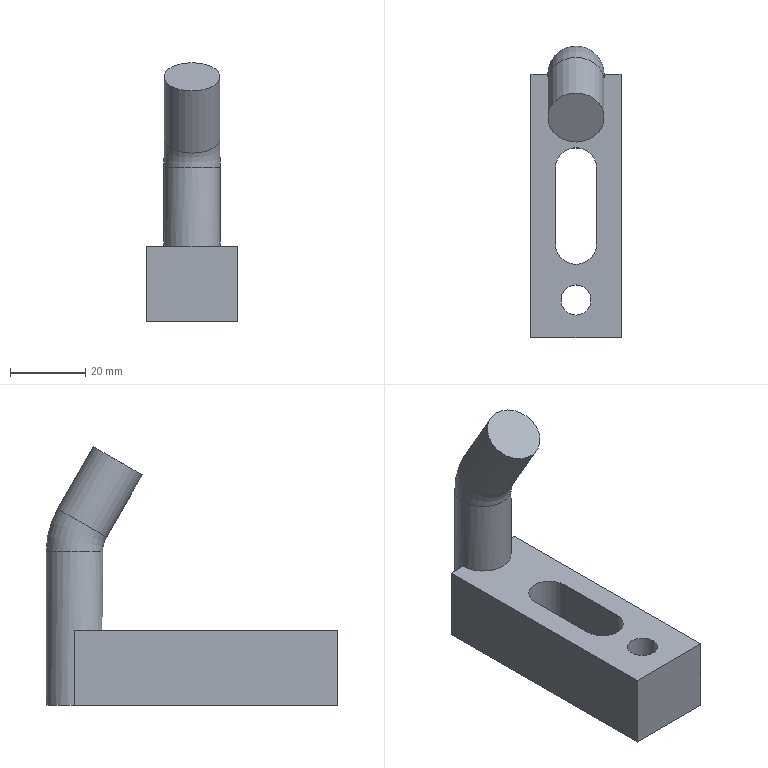Part | NX | features solid 2 | 1 solid | 16 faces | box 24 x 77.5 x 68.75 mm | volume 36527 mm3 | plane 10 | cylinder 5 | torus 1 | commonest cylinder face diameters 11 x2 15 x2 8 x1
STEP:
#1=CARTESIAN_POINT('',(-340.,270.,5.));
#2=VERTEX_POINT('',#1);
#3=CARTESIAN_POINT('',(-340.,266.,5.));
#4=DIRECTION('',(0.,0.,-1.));
#5=DIRECTION('',(0.,1.,0.));
#6=AXIS2_PLACEMENT_3D('',#3,#4,#5);
#7=CIRCLE('',#6,4.);
#8=EDGE_CURVE('',#2,#2,#7,.T.);
#9=ORIENTED_EDGE('',*,*,#8,.T.);
#10=EDGE_LOOP('',(#9));
#11=FACE_BOUND('',#10,.T.);
#12=CARTESIAN_POINT('',(-334.5,301.,5.));
#13=VERTEX_POINT('',#12);
#14=CARTESIAN_POINT('',(-334.5,281.,5.));
#15=VERTEX_POINT('',#14);
#16=CARTESIAN_POINT('',(-334.5,291.,5.));
#17=DIRECTION('',(0.,-1.,0.));
#18=VECTOR('',#17,1000.);
#19=LINE('',#16,#18);
#20=EDGE_CURVE('',#13,#15,#19,.T.);
#21=ORIENTED_EDGE('',*,*,#20,.T.);
#22=CARTESIAN_POINT('',(-345.5,281.,5.));
#23=VERTEX_POINT('',#22);
#24=CARTESIAN_POINT('',(-340.,281.,5.));
#25=DIRECTION('',(0.,0.,1.));
#26=DIRECTION('',(0.,-1.,0.));
#27=AXIS2_PLACEMENT_3D('',#24,#25,#26);
#28=CIRCLE('',#27,5.5);
#29=EDGE_CURVE('',#23,#15,#28,.T.);
#30=ORIENTED_EDGE('',*,*,#29,.F.);
#31=CARTESIAN_POINT('',(-345.5,301.,5.));
#32=VERTEX_POINT('',#31);
#33=CARTESIAN_POINT('',(-345.5,291.,5.));
#34=DIRECTION('',(0.,-1.,0.));
#35=VECTOR('',#34,1000.);
#36=LINE('',#33,#35);
#37=EDGE_CURVE('',#32,#23,#36,.T.);
#38=ORIENTED_EDGE('',*,*,#37,.F.);
#39=CARTESIAN_POINT('',(-340.,301.,5.));
#40=DIRECTION('',(0.,0.,1.));
#41=DIRECTION('',(0.,-1.,0.));
#42=AXIS2_PLACEMENT_3D('',#39,#40,#41);
#43=CIRCLE('',#42,5.5);
#44=EDGE_CURVE('',#13,#32,#43,.T.);
#45=ORIENTED_EDGE('',*,*,#44,.F.);
#46=EDGE_LOOP('',(#21,#30,#38,#45));
#47=FACE_BOUND('',#46,.T.);
#48=CARTESIAN_POINT('',(-328.,326.,5.));
#49=VERTEX_POINT('',#48);
#50=CARTESIAN_POINT('',(-332.5,326.,5.));
#51=VERTEX_POINT('',#50);
#52=CARTESIAN_POINT('',(-328.,326.,5.));
#53=DIRECTION('',(-1.,0.,0.));
#54=VECTOR('',#53,1000.);
#55=LINE('',#52,#54);
#56=EDGE_CURVE('',#49,#51,#55,.T.);
#57=ORIENTED_EDGE('',*,*,#56,.T.);
#58=CARTESIAN_POINT('',(-347.5,326.,5.));
#59=VERTEX_POINT('',#58);
#60=CARTESIAN_POINT('',(-340.,326.,5.));
#61=DIRECTION('',(0.,0.,1.));
#62=DIRECTION('',(1.,0.,0.));
#63=AXIS2_PLACEMENT_3D('',#60,#61,#62);
#64=CIRCLE('',#63,7.5);
#65=EDGE_CURVE('',#51,#59,#64,.F.);
#66=ORIENTED_EDGE('',*,*,#65,.T.);
#67=CARTESIAN_POINT('',(-352.,326.,5.));
#68=VERTEX_POINT('',#67);
#69=CARTESIAN_POINT('',(-328.,326.,5.));
#70=DIRECTION('',(-1.,0.,0.));
#71=VECTOR('',#70,1000.);
#72=LINE('',#69,#71);
#73=EDGE_CURVE('',#59,#68,#72,.T.);
#74=ORIENTED_EDGE('',*,*,#73,.T.);
#75=CARTESIAN_POINT('',(-352.,256.,5.));
#76=VERTEX_POINT('',#75);
#77=CARTESIAN_POINT('',(-352.,326.,5.));
#78=DIRECTION('',(0.,-1.,0.));
#79=VECTOR('',#78,1000.);
#80=LINE('',#77,#79);
#81=EDGE_CURVE('',#68,#76,#80,.T.);
#82=ORIENTED_EDGE('',*,*,#81,.T.);
#83=CARTESIAN_POINT('',(-328.,256.,5.));
#84=VERTEX_POINT('',#83);
#85=CARTESIAN_POINT('',(-352.,256.,5.));
#86=DIRECTION('',(1.,0.,0.));
#87=VECTOR('',#86,1000.);
#88=LINE('',#85,#87);
#89=EDGE_CURVE('',#76,#84,#88,.T.);
#90=ORIENTED_EDGE('',*,*,#89,.T.);
#91=CARTESIAN_POINT('',(-328.,256.,5.));
#92=DIRECTION('',(0.,1.,0.));
#93=VECTOR('',#92,1000.);
#94=LINE('',#91,#93);
#95=EDGE_CURVE('',#84,#49,#94,.T.);
#96=ORIENTED_EDGE('',*,*,#95,.T.);
#97=EDGE_LOOP('',(#57,#66,#74,#82,#90,#96));
#98=FACE_BOUND('',#97,.T.);
#99=CARTESIAN_POINT('',(-328.,256.,5.));
#100=DIRECTION('',(0.,0.,1.));
#101=DIRECTION('',(0.,-1.,0.));
#102=AXIS2_PLACEMENT_3D('',#99,#100,#101);
#103=PLANE('',#102);
#104=ADVANCED_FACE('',(#11,#47,#98),#103,.T.);
#105=CARTESIAN_POINT('',(-347.5,326.,-15.));
#106=VERTEX_POINT('',#105);
#107=CARTESIAN_POINT('',(-352.,326.,-15.));
#108=VERTEX_POINT('',#107);
#109=CARTESIAN_POINT('',(-328.,326.,-15.));
#110=DIRECTION('',(-1.,0.,0.));
#111=VECTOR('',#110,1000.);
#112=LINE('',#109,#111);
#113=EDGE_CURVE('',#106,#108,#112,.T.);
#114=ORIENTED_EDGE('',*,*,#113,.F.);
#115=CARTESIAN_POINT('',(-332.5,326.,-15.));
#116=VERTEX_POINT('',#115);
#117=CARTESIAN_POINT('',(-340.,326.,-15.));
#118=DIRECTION('',(0.,0.,1.));
#119=DIRECTION('',(0.,-1.,0.));
#120=AXIS2_PLACEMENT_3D('',#117,#118,#119);
#121=CIRCLE('',#120,7.5);
#122=EDGE_CURVE('',#116,#106,#121,.T.);
#123=ORIENTED_EDGE('',*,*,#122,.F.);
#124=CARTESIAN_POINT('',(-328.,326.,-15.));
#125=VERTEX_POINT('',#124);
#126=CARTESIAN_POINT('',(-328.,326.,-15.));
#127=DIRECTION('',(-1.,0.,0.));
#128=VECTOR('',#127,1000.);
#129=LINE('',#126,#128);
#130=EDGE_CURVE('',#125,#116,#129,.T.);
#131=ORIENTED_EDGE('',*,*,#130,.F.);
#132=CARTESIAN_POINT('',(-328.,256.,-15.));
#133=VERTEX_POINT('',#132);
#134=CARTESIAN_POINT('',(-328.,256.,-15.));
#135=DIRECTION('',(0.,1.,0.));
#136=VECTOR('',#135,1000.);
#137=LINE('',#134,#136);
#138=EDGE_CURVE('',#133,#125,#137,.T.);
#139=ORIENTED_EDGE('',*,*,#138,.F.);
#140=CARTESIAN_POINT('',(-352.,256.,-15.));
#141=VERTEX_POINT('',#140);
#142=CARTESIAN_POINT('',(-352.,256.,-15.));
#143=DIRECTION('',(1.,0.,0.));
#144=VECTOR('',#143,1000.);
#145=LINE('',#142,#144);
#146=EDGE_CURVE('',#141,#133,#145,.T.);
#147=ORIENTED_EDGE('',*,*,#146,.F.);
#148=CARTESIAN_POINT('',(-352.,326.,-15.));
#149=DIRECTION('',(0.,-1.,0.));
#150=VECTOR('',#149,1000.);
#151=LINE('',#148,#150);
#152=EDGE_CURVE('',#108,#141,#151,.T.);
#153=ORIENTED_EDGE('',*,*,#152,.F.);
#154=EDGE_LOOP('',(#114,#123,#131,#139,#147,#153));
#155=FACE_BOUND('',#154,.T.);
#156=CARTESIAN_POINT('',(-345.5,281.,-15.));
#157=VERTEX_POINT('',#156);
#158=CARTESIAN_POINT('',(-334.5,281.,-15.));
#159=VERTEX_POINT('',#158);
#160=CARTESIAN_POINT('',(-340.,281.,-15.));
#161=DIRECTION('',(0.,0.,1.));
#162=DIRECTION('',(0.,-1.,0.));
#163=AXIS2_PLACEMENT_3D('',#160,#161,#162);
#164=CIRCLE('',#163,5.5);
#165=EDGE_CURVE('',#157,#159,#164,.T.);
#166=ORIENTED_EDGE('',*,*,#165,.T.);
#167=CARTESIAN_POINT('',(-334.5,301.,-15.));
#168=VERTEX_POINT('',#167);
#169=CARTESIAN_POINT('',(-334.5,301.,-15.));
#170=DIRECTION('',(0.,-1.,0.));
#171=VECTOR('',#170,1000.);
#172=LINE('',#169,#171);
#173=EDGE_CURVE('',#168,#159,#172,.T.);
#174=ORIENTED_EDGE('',*,*,#173,.F.);
#175=CARTESIAN_POINT('',(-345.5,301.,-15.));
#176=VERTEX_POINT('',#175);
#177=CARTESIAN_POINT('',(-340.,301.,-15.));
#178=DIRECTION('',(0.,0.,1.));
#179=DIRECTION('',(0.,-1.,0.));
#180=AXIS2_PLACEMENT_3D('',#177,#178,#179);
#181=CIRCLE('',#180,5.5);
#182=EDGE_CURVE('',#168,#176,#181,.T.);
#183=ORIENTED_EDGE('',*,*,#182,.T.);
#184=CARTESIAN_POINT('',(-345.5,301.,-15.));
#185=DIRECTION('',(0.,-1.,0.));
#186=VECTOR('',#185,1000.);
#187=LINE('',#184,#186);
#188=EDGE_CURVE('',#176,#157,#187,.T.);
#189=ORIENTED_EDGE('',*,*,#188,.T.);
#190=EDGE_LOOP('',(#166,#174,#183,#189));
#191=FACE_BOUND('',#190,.T.);
#192=CARTESIAN_POINT('',(-340.,262.,-15.));
#193=VERTEX_POINT('',#192);
#194=CARTESIAN_POINT('',(-340.,266.,-15.));
#195=DIRECTION('',(0.,0.,1.));
#196=DIRECTION('',(0.,-1.,0.));
#197=AXIS2_PLACEMENT_3D('',#194,#195,#196);
#198=CIRCLE('',#197,4.);
#199=EDGE_CURVE('',#193,#193,#198,.T.);
#200=ORIENTED_EDGE('',*,*,#199,.T.);
#201=EDGE_LOOP('',(#200));
#202=FACE_BOUND('',#201,.T.);
#203=CARTESIAN_POINT('',(-328.,256.,-15.));
#204=DIRECTION('',(0.,0.,1.));
#205=DIRECTION('',(0.,-1.,0.));
#206=AXIS2_PLACEMENT_3D('',#203,#204,#205);
#207=PLANE('',#206);
#208=ADVANCED_FACE('',(#155,#191,#202),#207,.F.);
#209=ORIENTED_EDGE('',*,*,#138,.T.);
#210=CARTESIAN_POINT('',(-328.,326.,5.));
#211=DIRECTION('',(0.,0.,-1.));
#212=VECTOR('',#211,1000.);
#213=LINE('',#210,#212);
#214=EDGE_CURVE('',#49,#125,#213,.T.);
#215=ORIENTED_EDGE('',*,*,#214,.F.);
#216=ORIENTED_EDGE('',*,*,#95,.F.);
#217=CARTESIAN_POINT('',(-328.,256.,5.));
#218=DIRECTION('',(0.,0.,-1.));
#219=VECTOR('',#218,1000.);
#220=LINE('',#217,#219);
#221=EDGE_CURVE('',#84,#133,#220,.T.);
#222=ORIENTED_EDGE('',*,*,#221,.T.);
#223=EDGE_LOOP('',(#209,#215,#216,#222));
#224=FACE_BOUND('',#223,.T.);
#225=CARTESIAN_POINT('',(-328.,256.,5.));
#226=DIRECTION('',(-1.,0.,0.));
#227=DIRECTION('',(0.,-1.,0.));
#228=AXIS2_PLACEMENT_3D('',#225,#226,#227);
#229=PLANE('',#228);
#230=ADVANCED_FACE('',(#224),#229,.F.);
#231=ORIENTED_EDGE('',*,*,#146,.T.);
#232=ORIENTED_EDGE('',*,*,#221,.F.);
#233=ORIENTED_EDGE('',*,*,#89,.F.);
#234=CARTESIAN_POINT('',(-352.,256.,5.));
#235=DIRECTION('',(0.,0.,-1.));
#236=VECTOR('',#235,1000.);
#237=LINE('',#234,#236);
#238=EDGE_CURVE('',#76,#141,#237,.T.);
#239=ORIENTED_EDGE('',*,*,#238,.T.);
#240=EDGE_LOOP('',(#231,#232,#233,#239));
#241=FACE_BOUND('',#240,.T.);
#242=CARTESIAN_POINT('',(-352.,256.,5.));
#243=DIRECTION('',(0.,1.,0.));
#244=DIRECTION('',(0.,0.,1.));
#245=AXIS2_PLACEMENT_3D('',#242,#243,#244);
#246=PLANE('',#245);
#247=ADVANCED_FACE('',(#241),#246,.F.);
#248=ORIENTED_EDGE('',*,*,#152,.T.);
#249=ORIENTED_EDGE('',*,*,#238,.F.);
#250=ORIENTED_EDGE('',*,*,#81,.F.);
#251=CARTESIAN_POINT('',(-352.,326.,5.));
#252=DIRECTION('',(0.,0.,-1.));
#253=VECTOR('',#252,1000.);
#254=LINE('',#251,#253);
#255=EDGE_CURVE('',#68,#108,#254,.T.);
#256=ORIENTED_EDGE('',*,*,#255,.T.);
#257=EDGE_LOOP('',(#248,#249,#250,#256));
#258=FACE_BOUND('',#257,.T.);
#259=CARTESIAN_POINT('',(-352.,326.,5.));
#260=DIRECTION('',(1.,0.,0.));
#261=DIRECTION('',(0.,1.,0.));
#262=AXIS2_PLACEMENT_3D('',#259,#260,#261);
#263=PLANE('',#262);
#264=ADVANCED_FACE('',(#258),#263,.F.);
#265=CARTESIAN_POINT('',(-347.5,326.,40.981));
#266=DIRECTION('',(0.,0.,-1.));
#267=VECTOR('',#266,1000.);
#268=LINE('',#265,#267);
#269=EDGE_CURVE('',#106,#59,#268,.F.);
#270=ORIENTED_EDGE('',*,*,#269,.F.);
#271=ORIENTED_EDGE('',*,*,#113,.T.);
#272=ORIENTED_EDGE('',*,*,#255,.F.);
#273=ORIENTED_EDGE('',*,*,#73,.F.);
#274=EDGE_LOOP('',(#270,#271,#272,#273));
#275=FACE_BOUND('',#274,.T.);
#276=CARTESIAN_POINT('',(-328.,326.,5.));
#277=DIRECTION('',(0.,-1.,0.));
#278=DIRECTION('',(0.,0.,-1.));
#279=AXIS2_PLACEMENT_3D('',#276,#277,#278);
#280=PLANE('',#279);
#281=ADVANCED_FACE('',(#275),#280,.F.);
#282=CARTESIAN_POINT('',(-332.5,326.,40.981));
#283=DIRECTION('',(0.,0.,-1.));
#284=VECTOR('',#283,1000.);
#285=LINE('',#282,#284);
#286=EDGE_CURVE('',#51,#116,#285,.T.);
#287=ORIENTED_EDGE('',*,*,#286,.T.);
#288=ORIENTED_EDGE('',*,*,#122,.T.);
#289=ORIENTED_EDGE('',*,*,#269,.T.);
#290=ORIENTED_EDGE('',*,*,#65,.F.);
#291=EDGE_LOOP('',(#287,#288,#289,#290));
#292=FACE_BOUND('',#291,.T.);
#293=CARTESIAN_POINT('',(-340.,318.5,25.981));
#294=VERTEX_POINT('',#293);
#295=CARTESIAN_POINT('',(-340.,326.,25.981));
#296=DIRECTION('',(0.,0.,1.));
#297=DIRECTION('',(0.,-1.,0.));
#298=AXIS2_PLACEMENT_3D('',#295,#296,#297);
#299=CIRCLE('',#298,7.5);
#300=EDGE_CURVE('',#294,#294,#299,.T.);
#301=ORIENTED_EDGE('',*,*,#300,.F.);
#302=EDGE_LOOP('',(#301));
#303=FACE_BOUND('',#302,.T.);
#304=CARTESIAN_POINT('',(-340.,326.,40.981));
#305=DIRECTION('',(0.,0.,-1.));
#306=DIRECTION('',(0.,1.,0.));
#307=AXIS2_PLACEMENT_3D('',#304,#305,#306);
#308=CYLINDRICAL_SURFACE('',#307,7.5);
#309=ADVANCED_FACE('',(#292,#303),#308,.T.);
#310=ORIENTED_EDGE('',*,*,#286,.F.);
#311=ORIENTED_EDGE('',*,*,#56,.F.);
#312=ORIENTED_EDGE('',*,*,#214,.T.);
#313=ORIENTED_EDGE('',*,*,#130,.T.);
#314=EDGE_LOOP('',(#310,#311,#312,#313));
#315=FACE_BOUND('',#314,.T.);
#316=CARTESIAN_POINT('',(-328.,326.,5.));
#317=DIRECTION('',(0.,-1.,0.));
#318=DIRECTION('',(0.,0.,-1.));
#319=AXIS2_PLACEMENT_3D('',#316,#317,#318);
#320=PLANE('',#319);
#321=ADVANCED_FACE('',(#315),#320,.F.);
#322=ORIENTED_EDGE('',*,*,#8,.F.);
#323=EDGE_LOOP('',(#322));
#324=FACE_BOUND('',#323,.T.);
#325=ORIENTED_EDGE('',*,*,#199,.F.);
#326=EDGE_LOOP('',(#325));
#327=FACE_BOUND('',#326,.T.);
#328=CARTESIAN_POINT('',(-340.,266.,5.));
#329=DIRECTION('',(0.,0.,-1.));
#330=DIRECTION('',(0.,1.,0.));
#331=AXIS2_PLACEMENT_3D('',#328,#329,#330);
#332=CYLINDRICAL_SURFACE('',#331,4.);
#333=ADVANCED_FACE('',(#324,#327),#332,.F.);
#334=ORIENTED_EDGE('',*,*,#44,.T.);
#335=CARTESIAN_POINT('',(-345.5,301.,5.));
#336=DIRECTION('',(0.,0.,1.));
#337=VECTOR('',#336,1000.);
#338=LINE('',#335,#337);
#339=EDGE_CURVE('',#176,#32,#338,.T.);
#340=ORIENTED_EDGE('',*,*,#339,.F.);
#341=ORIENTED_EDGE('',*,*,#182,.F.);
#342=CARTESIAN_POINT('',(-334.5,301.,5.));
#343=DIRECTION('',(0.,0.,1.));
#344=VECTOR('',#343,1000.);
#345=LINE('',#342,#344);
#346=EDGE_CURVE('',#168,#13,#345,.T.);
#347=ORIENTED_EDGE('',*,*,#346,.T.);
#348=EDGE_LOOP('',(#334,#340,#341,#347));
#349=FACE_BOUND('',#348,.T.);
#350=CARTESIAN_POINT('',(-340.,301.,5.));
#351=DIRECTION('',(0.,0.,1.));
#352=DIRECTION('',(0.,-1.,0.));
#353=AXIS2_PLACEMENT_3D('',#350,#351,#352);
#354=CYLINDRICAL_SURFACE('',#353,5.5);
#355=ADVANCED_FACE('',(#349),#354,.F.);
#356=ORIENTED_EDGE('',*,*,#37,.T.);
#357=CARTESIAN_POINT('',(-345.5,281.,5.));
#358=DIRECTION('',(0.,0.,1.));
#359=VECTOR('',#358,1000.);
#360=LINE('',#357,#359);
#361=EDGE_CURVE('',#157,#23,#360,.T.);
#362=ORIENTED_EDGE('',*,*,#361,.F.);
#363=ORIENTED_EDGE('',*,*,#188,.F.);
#364=ORIENTED_EDGE('',*,*,#339,.T.);
#365=EDGE_LOOP('',(#356,#362,#363,#364));
#366=FACE_BOUND('',#365,.T.);
#367=CARTESIAN_POINT('',(-345.5,291.,5.));
#368=DIRECTION('',(-1.,0.,0.));
#369=DIRECTION('',(0.,0.,-1.));
#370=AXIS2_PLACEMENT_3D('',#367,#368,#369);
#371=PLANE('',#370);
#372=ADVANCED_FACE('',(#366),#371,.F.);
#373=ORIENTED_EDGE('',*,*,#29,.T.);
#374=CARTESIAN_POINT('',(-334.5,281.,5.));
#375=DIRECTION('',(0.,0.,1.));
#376=VECTOR('',#375,1000.);
#377=LINE('',#374,#376);
#378=EDGE_CURVE('',#159,#15,#377,.T.);
#379=ORIENTED_EDGE('',*,*,#378,.F.);
#380=ORIENTED_EDGE('',*,*,#165,.F.);
#381=ORIENTED_EDGE('',*,*,#361,.T.);
#382=EDGE_LOOP('',(#373,#379,#380,#381));
#383=FACE_BOUND('',#382,.T.);
#384=CARTESIAN_POINT('',(-340.,281.,5.));
#385=DIRECTION('',(0.,0.,1.));
#386=DIRECTION('',(0.,-1.,0.));
#387=AXIS2_PLACEMENT_3D('',#384,#385,#386);
#388=CYLINDRICAL_SURFACE('',#387,5.5);
#389=ADVANCED_FACE('',(#383),#388,.F.);
#390=ORIENTED_EDGE('',*,*,#20,.F.);
#391=ORIENTED_EDGE('',*,*,#346,.F.);
#392=ORIENTED_EDGE('',*,*,#173,.T.);
#393=ORIENTED_EDGE('',*,*,#378,.T.);
#394=EDGE_LOOP('',(#390,#391,#392,#393));
#395=FACE_BOUND('',#394,.T.);
#396=CARTESIAN_POINT('',(-334.5,291.,5.));
#397=DIRECTION('',(1.,0.,0.));
#398=DIRECTION('',(0.,0.,1.));
#399=AXIS2_PLACEMENT_3D('',#396,#397,#398);
#400=PLANE('',#399);
#401=ADVANCED_FACE('',(#395),#400,.F.);
#402=CARTESIAN_POINT('',(-340.,317.495,29.731));
#403=VERTEX_POINT('',#402);
#404=CARTESIAN_POINT('',(-340.,323.99,33.481));
#405=DIRECTION('',(0.,-0.5,0.866));
#406=DIRECTION('',(0.,-0.866,-0.5));
#407=AXIS2_PLACEMENT_3D('',#404,#405,#406);
#408=CIRCLE('',#407,7.5);
#409=EDGE_CURVE('',#403,#403,#408,.T.);
#410=ORIENTED_EDGE('',*,*,#409,.T.);
#411=EDGE_LOOP('',(#410));
#412=FACE_BOUND('',#411,.T.);
#413=CARTESIAN_POINT('',(-340.,307.958,46.25));
#414=VERTEX_POINT('',#413);
#415=CARTESIAN_POINT('',(-340.,314.453,50.));
#416=DIRECTION('',(0.,-0.5,0.866));
#417=DIRECTION('',(0.,-0.866,-0.5));
#418=AXIS2_PLACEMENT_3D('',#415,#416,#417);
#419=CIRCLE('',#418,7.5);
#420=EDGE_CURVE('',#414,#414,#419,.T.);
#421=ORIENTED_EDGE('',*,*,#420,.F.);
#422=EDGE_LOOP('',(#421));
#423=FACE_BOUND('',#422,.T.);
#424=CARTESIAN_POINT('',(-340.,323.99,33.481));
#425=DIRECTION('',(0.,-0.5,0.866));
#426=DIRECTION('',(0.,-0.866,-0.5));
#427=AXIS2_PLACEMENT_3D('',#424,#425,#426);
#428=CYLINDRICAL_SURFACE('',#427,7.5);
#429=ADVANCED_FACE('',(#412,#423),#428,.T.);
#430=ORIENTED_EDGE('',*,*,#300,.T.);
#431=EDGE_LOOP('',(#430));
#432=FACE_BOUND('',#431,.T.);
#433=ORIENTED_EDGE('',*,*,#409,.F.);
#434=EDGE_LOOP('',(#433));
#435=FACE_BOUND('',#434,.T.);
#436=CARTESIAN_POINT('',(-340.,311.,25.981));
#437=DIRECTION('',(1.,0.,0.));
#438=DIRECTION('',(0.,0.,1.));
#439=AXIS2_PLACEMENT_3D('',#436,#437,#438);
#440=TOROIDAL_SURFACE('',#439,15.,7.5);
#441=ADVANCED_FACE('',(#432,#435),#440,.T.);
#442=ORIENTED_EDGE('',*,*,#420,.T.);
#443=EDGE_LOOP('',(#442));
#444=FACE_BOUND('',#443,.T.);
#445=CARTESIAN_POINT('',(-340.,314.453,50.));
#446=DIRECTION('',(0.,-0.5,0.866));
#447=DIRECTION('',(0.,-0.866,-0.5));
#448=AXIS2_PLACEMENT_3D('',#445,#446,#447);
#449=PLANE('',#448);
#450=ADVANCED_FACE('',(#444),#449,.T.);
#451=CLOSED_SHELL('',(#104,#208,#230,#247,#264,#281,#309,#321,#333,#355,#372,#389,#401,#429,#441,#450));
#452=MANIFOLD_SOLID_BREP('',#451);
#453=(LENGTH_UNIT()NAMED_UNIT(*)SI_UNIT(.MILLI.,.METRE.));
#454=UNCERTAINTY_MEASURE_WITH_UNIT(LENGTH_MEASURE(0.00001),#453,'','');
#455=(NAMED_UNIT(*)PLANE_ANGLE_UNIT()SI_UNIT($,.RADIAN.));
#456=(NAMED_UNIT(*)SI_UNIT($,.STERADIAN.)SOLID_ANGLE_UNIT());
#457=(GEOMETRIC_REPRESENTATION_CONTEXT(3)GLOBAL_UNCERTAINTY_ASSIGNED_CONTEXT((#454))GLOBAL_UNIT_ASSIGNED_CONTEXT((#453,#455,#456))REPRESENTATION_CONTEXT('',''));
#458=ADVANCED_BREP_SHAPE_REPRESENTATION('',(#452),#457);